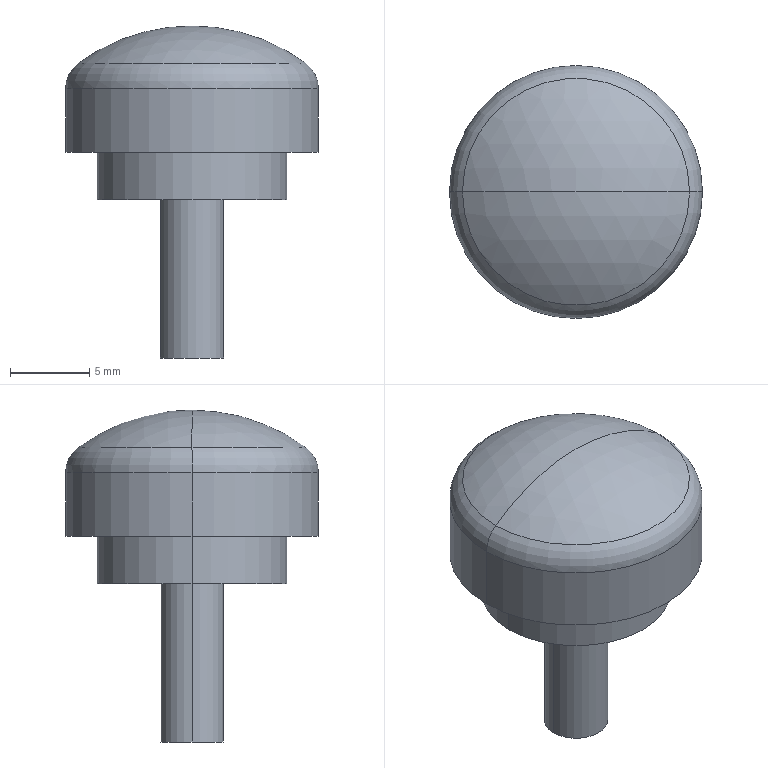Part | SolidWorks | features ICE 2, Dome 1, Extrusion 1, Fillet 1 | 1 solid | 13 faces | box 16 x 16 x 21 mm | volume 1779 mm3 | cylinder 6 | plane 3 | torus 2 | sphere 2 | commonest cylinder face diameters 4 x2 12 x2 16 x2
STEP:
#1=CARTESIAN_POINT('',(7.18,0.,18.655));
#2=VERTEX_POINT('',#1);
#3=CARTESIAN_POINT('',(-7.18,0.,18.655));
#4=VERTEX_POINT('',#3);
#5=CARTESIAN_POINT('',(0.,0.,18.655));
#6=DIRECTION('',(0.,0.,1.));
#7=DIRECTION('',(-1.,0.,0.));
#8=AXIS2_PLACEMENT_3D('',#5,#6,#7);
#9=CIRCLE('',#8,7.18);
#10=EDGE_CURVE('',#2,#4,#9,.T.);
#11=ORIENTED_EDGE('',*,*,#10,.F.);
#12=CARTESIAN_POINT('',(8.,0.,17.041));
#13=VERTEX_POINT('',#12);
#14=CARTESIAN_POINT('',(6.,0.,17.041));
#15=DIRECTION('',(0.,1.,0.));
#16=DIRECTION('',(-1.,0.,0.));
#17=AXIS2_PLACEMENT_3D('',#14,#15,#16);
#18=CIRCLE('',#17,2.);
#19=EDGE_CURVE('',#2,#13,#18,.T.);
#20=ORIENTED_EDGE('',*,*,#19,.T.);
#21=CARTESIAN_POINT('',(-8.,0.,17.041));
#22=VERTEX_POINT('',#21);
#23=CARTESIAN_POINT('',(0.,0.,17.041));
#24=DIRECTION('',(0.,0.,-1.));
#25=DIRECTION('',(-1.,0.,0.));
#26=AXIS2_PLACEMENT_3D('',#23,#24,#25);
#27=CIRCLE('',#26,8.);
#28=EDGE_CURVE('',#22,#13,#27,.T.);
#29=ORIENTED_EDGE('',*,*,#28,.F.);
#30=CARTESIAN_POINT('',(-6.,0.,17.041));
#31=DIRECTION('',(0.,-1.,0.));
#32=DIRECTION('',(0.,0.,-1.));
#33=AXIS2_PLACEMENT_3D('',#30,#31,#32);
#34=CIRCLE('',#33,2.);
#35=EDGE_CURVE('',#4,#22,#34,.T.);
#36=ORIENTED_EDGE('',*,*,#35,.F.);
#37=EDGE_LOOP('',(#11,#20,#29,#36));
#38=FACE_OUTER_BOUND('',#37,.T.);
#39=CARTESIAN_POINT('',(0.,0.,17.041));
#40=DIRECTION('',(0.,0.,-1.));
#41=DIRECTION('',(-1.,0.,0.));
#42=AXIS2_PLACEMENT_3D('',#39,#40,#41);
#43=TOROIDAL_SURFACE('',#42,6.,2.);
#44=ADVANCED_FACE('',(#38),#43,.T.);
#45=ORIENTED_EDGE('',*,*,#28,.T.);
#46=CARTESIAN_POINT('',(8.,0.,13.));
#47=VERTEX_POINT('',#46);
#48=CARTESIAN_POINT('',(8.,0.,18.));
#49=DIRECTION('',(0.,0.,-1.));
#50=VECTOR('',#49,1000.);
#51=LINE('',#48,#50);
#52=EDGE_CURVE('',#13,#47,#51,.T.);
#53=ORIENTED_EDGE('',*,*,#52,.T.);
#54=CARTESIAN_POINT('',(-8.,0.,13.));
#55=VERTEX_POINT('',#54);
#56=CARTESIAN_POINT('',(0.,0.,13.));
#57=DIRECTION('',(0.,0.,-1.));
#58=DIRECTION('',(-1.,0.,0.));
#59=AXIS2_PLACEMENT_3D('',#56,#57,#58);
#60=CIRCLE('',#59,8.);
#61=EDGE_CURVE('',#55,#47,#60,.T.);
#62=ORIENTED_EDGE('',*,*,#61,.F.);
#63=CARTESIAN_POINT('',(-8.,0.,18.));
#64=DIRECTION('',(0.,0.,-1.));
#65=VECTOR('',#64,1000.);
#66=LINE('',#63,#65);
#67=EDGE_CURVE('',#22,#55,#66,.T.);
#68=ORIENTED_EDGE('',*,*,#67,.F.);
#69=EDGE_LOOP('',(#45,#53,#62,#68));
#70=FACE_OUTER_BOUND('',#69,.T.);
#71=CARTESIAN_POINT('',(0.,0.,18.));
#72=DIRECTION('',(0.,0.,-1.));
#73=DIRECTION('',(-1.,0.,0.));
#74=AXIS2_PLACEMENT_3D('',#71,#72,#73);
#75=CYLINDRICAL_SURFACE('',#74,8.);
#76=ADVANCED_FACE('',(#70),#75,.T.);
#77=ORIENTED_EDGE('',*,*,#10,.T.);
#78=CARTESIAN_POINT('',(0.,0.,21.));
#79=VERTEX_POINT('',#78);
#80=CARTESIAN_POINT('',(0.,0.,8.833));
#81=DIRECTION('',(0.,1.,0.));
#82=DIRECTION('',(-1.,0.,0.));
#83=AXIS2_PLACEMENT_3D('',#80,#81,#82);
#84=CIRCLE('',#83,12.167);
#85=EDGE_CURVE('',#4,#79,#84,.T.);
#86=ORIENTED_EDGE('',*,*,#85,.T.);
#87=CARTESIAN_POINT('',(0.,0.,8.833));
#88=DIRECTION('',(0.,-1.,0.));
#89=DIRECTION('',(0.,0.,-1.));
#90=AXIS2_PLACEMENT_3D('',#87,#88,#89);
#91=CIRCLE('',#90,12.167);
#92=EDGE_CURVE('',#2,#79,#91,.T.);
#93=ORIENTED_EDGE('',*,*,#92,.F.);
#94=EDGE_LOOP('',(#77,#86,#93));
#95=FACE_OUTER_BOUND('',#94,.T.);
#96=CARTESIAN_POINT('',(0.,0.,8.833));
#97=DIRECTION('',(0.,1.,0.));
#98=DIRECTION('',(1.,0.,0.));
#99=AXIS2_PLACEMENT_3D('',#96,#97,#98);
#100=SPHERICAL_SURFACE('',#99,12.167);
#101=ADVANCED_FACE('',(#95),#100,.T.);
#102=CARTESIAN_POINT('',(-6.,0.,13.));
#103=VERTEX_POINT('',#102);
#104=CARTESIAN_POINT('',(6.,0.,13.));
#105=VERTEX_POINT('',#104);
#106=CARTESIAN_POINT('',(0.,0.,13.));
#107=DIRECTION('',(0.,0.,-1.));
#108=DIRECTION('',(-1.,0.,0.));
#109=AXIS2_PLACEMENT_3D('',#106,#107,#108);
#110=CIRCLE('',#109,6.);
#111=EDGE_CURVE('',#103,#105,#110,.T.);
#112=ORIENTED_EDGE('',*,*,#111,.T.);
#113=CARTESIAN_POINT('',(6.,0.,10.));
#114=VERTEX_POINT('',#113);
#115=CARTESIAN_POINT('',(6.,0.,13.));
#116=DIRECTION('',(0.,0.,-1.));
#117=VECTOR('',#116,1000.);
#118=LINE('',#115,#117);
#119=EDGE_CURVE('',#105,#114,#118,.T.);
#120=ORIENTED_EDGE('',*,*,#119,.T.);
#121=CARTESIAN_POINT('',(-6.,0.,10.));
#122=VERTEX_POINT('',#121);
#123=CARTESIAN_POINT('',(0.,0.,10.));
#124=DIRECTION('',(0.,0.,-1.));
#125=DIRECTION('',(-1.,0.,0.));
#126=AXIS2_PLACEMENT_3D('',#123,#124,#125);
#127=CIRCLE('',#126,6.);
#128=EDGE_CURVE('',#122,#114,#127,.T.);
#129=ORIENTED_EDGE('',*,*,#128,.F.);
#130=CARTESIAN_POINT('',(-6.,0.,13.));
#131=DIRECTION('',(0.,0.,-1.));
#132=VECTOR('',#131,1000.);
#133=LINE('',#130,#132);
#134=EDGE_CURVE('',#103,#122,#133,.T.);
#135=ORIENTED_EDGE('',*,*,#134,.F.);
#136=EDGE_LOOP('',(#112,#120,#129,#135));
#137=FACE_OUTER_BOUND('',#136,.T.);
#138=CARTESIAN_POINT('',(0.,0.,13.));
#139=DIRECTION('',(0.,0.,-1.));
#140=DIRECTION('',(-1.,0.,0.));
#141=AXIS2_PLACEMENT_3D('',#138,#139,#140);
#142=CYLINDRICAL_SURFACE('',#141,6.);
#143=ADVANCED_FACE('',(#137),#142,.T.);
#144=CARTESIAN_POINT('',(2.,0.,10.));
#145=VERTEX_POINT('',#144);
#146=CARTESIAN_POINT('',(-2.,0.,10.));
#147=VERTEX_POINT('',#146);
#148=CARTESIAN_POINT('',(0.,0.,10.));
#149=DIRECTION('',(0.,0.,1.));
#150=DIRECTION('',(1.,0.,0.));
#151=AXIS2_PLACEMENT_3D('',#148,#149,#150);
#152=CIRCLE('',#151,2.);
#153=EDGE_CURVE('',#145,#147,#152,.T.);
#154=ORIENTED_EDGE('',*,*,#153,.F.);
#155=CARTESIAN_POINT('',(2.,0.,0.));
#156=VERTEX_POINT('',#155);
#157=CARTESIAN_POINT('',(2.,0.,10.));
#158=DIRECTION('',(0.,0.,-1.));
#159=VECTOR('',#158,1000.);
#160=LINE('',#157,#159);
#161=EDGE_CURVE('',#145,#156,#160,.T.);
#162=ORIENTED_EDGE('',*,*,#161,.T.);
#163=CARTESIAN_POINT('',(-2.,0.,0.));
#164=VERTEX_POINT('',#163);
#165=CARTESIAN_POINT('',(0.,0.,0.));
#166=DIRECTION('',(0.,0.,1.));
#167=DIRECTION('',(1.,0.,0.));
#168=AXIS2_PLACEMENT_3D('',#165,#166,#167);
#169=CIRCLE('',#168,2.);
#170=EDGE_CURVE('',#156,#164,#169,.T.);
#171=ORIENTED_EDGE('',*,*,#170,.T.);
#172=CARTESIAN_POINT('',(-2.,0.,10.));
#173=DIRECTION('',(0.,0.,-1.));
#174=VECTOR('',#173,1000.);
#175=LINE('',#172,#174);
#176=EDGE_CURVE('',#147,#164,#175,.T.);
#177=ORIENTED_EDGE('',*,*,#176,.F.);
#178=EDGE_LOOP('',(#154,#162,#171,#177));
#179=FACE_OUTER_BOUND('',#178,.T.);
#180=CARTESIAN_POINT('',(0.,0.,10.));
#181=DIRECTION('',(0.,0.,-1.));
#182=DIRECTION('',(-1.,0.,0.));
#183=AXIS2_PLACEMENT_3D('',#180,#181,#182);
#184=CYLINDRICAL_SURFACE('',#183,2.);
#185=ADVANCED_FACE('',(#179),#184,.T.);
#186=CARTESIAN_POINT('',(0.,0.,10.));
#187=DIRECTION('',(0.,0.,1.));
#188=DIRECTION('',(1.,0.,0.));
#189=AXIS2_PLACEMENT_3D('',#186,#187,#188);
#190=CIRCLE('',#189,2.);
#191=EDGE_CURVE('',#147,#145,#190,.T.);
#192=ORIENTED_EDGE('',*,*,#191,.T.);
#193=ORIENTED_EDGE('',*,*,#153,.T.);
#194=EDGE_LOOP('',(#192,#193));
#195=FACE_BOUND('',#194,.T.);
#196=ORIENTED_EDGE('',*,*,#128,.T.);
#197=CARTESIAN_POINT('',(0.,0.,10.));
#198=DIRECTION('',(0.,0.,-1.));
#199=DIRECTION('',(-1.,0.,0.));
#200=AXIS2_PLACEMENT_3D('',#197,#198,#199);
#201=CIRCLE('',#200,6.);
#202=EDGE_CURVE('',#114,#122,#201,.T.);
#203=ORIENTED_EDGE('',*,*,#202,.T.);
#204=EDGE_LOOP('',(#196,#203));
#205=FACE_OUTER_BOUND('',#204,.T.);
#206=CARTESIAN_POINT('',(0.,0.,10.));
#207=DIRECTION('',(0.,0.,1.));
#208=DIRECTION('',(1.,0.,0.));
#209=AXIS2_PLACEMENT_3D('',#206,#207,#208);
#210=PLANE('',#209);
#211=ADVANCED_FACE('',(#195,#205),#210,.F.);
#212=ORIENTED_EDGE('',*,*,#161,.F.);
#213=ORIENTED_EDGE('',*,*,#191,.F.);
#214=ORIENTED_EDGE('',*,*,#176,.T.);
#215=CARTESIAN_POINT('',(0.,0.,0.));
#216=DIRECTION('',(0.,0.,1.));
#217=DIRECTION('',(1.,0.,0.));
#218=AXIS2_PLACEMENT_3D('',#215,#216,#217);
#219=CIRCLE('',#218,2.);
#220=EDGE_CURVE('',#164,#156,#219,.T.);
#221=ORIENTED_EDGE('',*,*,#220,.T.);
#222=EDGE_LOOP('',(#212,#213,#214,#221));
#223=FACE_OUTER_BOUND('',#222,.T.);
#224=CARTESIAN_POINT('',(0.,0.,10.));
#225=DIRECTION('',(0.,0.,-1.));
#226=DIRECTION('',(-1.,0.,0.));
#227=AXIS2_PLACEMENT_3D('',#224,#225,#226);
#228=CYLINDRICAL_SURFACE('',#227,2.);
#229=ADVANCED_FACE('',(#223),#228,.T.);
#230=ORIENTED_EDGE('',*,*,#220,.F.);
#231=ORIENTED_EDGE('',*,*,#170,.F.);
#232=EDGE_LOOP('',(#230,#231));
#233=FACE_OUTER_BOUND('',#232,.T.);
#234=CARTESIAN_POINT('',(0.,0.,0.));
#235=DIRECTION('',(0.,0.,1.));
#236=DIRECTION('',(1.,0.,0.));
#237=AXIS2_PLACEMENT_3D('',#234,#235,#236);
#238=PLANE('',#237);
#239=ADVANCED_FACE('',(#233),#238,.F.);
#240=ORIENTED_EDGE('',*,*,#111,.F.);
#241=CARTESIAN_POINT('',(0.,0.,13.));
#242=DIRECTION('',(0.,0.,-1.));
#243=DIRECTION('',(-1.,0.,0.));
#244=AXIS2_PLACEMENT_3D('',#241,#242,#243);
#245=CIRCLE('',#244,6.);
#246=EDGE_CURVE('',#105,#103,#245,.T.);
#247=ORIENTED_EDGE('',*,*,#246,.F.);
#248=EDGE_LOOP('',(#240,#247));
#249=FACE_BOUND('',#248,.T.);
#250=ORIENTED_EDGE('',*,*,#61,.T.);
#251=CARTESIAN_POINT('',(0.,0.,13.));
#252=DIRECTION('',(0.,0.,-1.));
#253=DIRECTION('',(-1.,0.,0.));
#254=AXIS2_PLACEMENT_3D('',#251,#252,#253);
#255=CIRCLE('',#254,8.);
#256=EDGE_CURVE('',#47,#55,#255,.T.);
#257=ORIENTED_EDGE('',*,*,#256,.T.);
#258=EDGE_LOOP('',(#250,#257));
#259=FACE_OUTER_BOUND('',#258,.T.);
#260=CARTESIAN_POINT('',(0.,0.,13.));
#261=DIRECTION('',(0.,0.,-1.));
#262=DIRECTION('',(-1.,0.,0.));
#263=AXIS2_PLACEMENT_3D('',#260,#261,#262);
#264=PLANE('',#263);
#265=ADVANCED_FACE('',(#249,#259),#264,.T.);
#266=ORIENTED_EDGE('',*,*,#119,.F.);
#267=ORIENTED_EDGE('',*,*,#246,.T.);
#268=ORIENTED_EDGE('',*,*,#134,.T.);
#269=ORIENTED_EDGE('',*,*,#202,.F.);
#270=EDGE_LOOP('',(#266,#267,#268,#269));
#271=FACE_OUTER_BOUND('',#270,.T.);
#272=CARTESIAN_POINT('',(0.,0.,13.));
#273=DIRECTION('',(0.,0.,-1.));
#274=DIRECTION('',(-1.,0.,0.));
#275=AXIS2_PLACEMENT_3D('',#272,#273,#274);
#276=CYLINDRICAL_SURFACE('',#275,6.);
#277=ADVANCED_FACE('',(#271),#276,.T.);
#278=ORIENTED_EDGE('',*,*,#85,.F.);
#279=CARTESIAN_POINT('',(0.,0.,18.655));
#280=DIRECTION('',(0.,0.,1.));
#281=DIRECTION('',(-1.,0.,0.));
#282=AXIS2_PLACEMENT_3D('',#279,#280,#281);
#283=CIRCLE('',#282,7.18);
#284=EDGE_CURVE('',#4,#2,#283,.T.);
#285=ORIENTED_EDGE('',*,*,#284,.T.);
#286=ORIENTED_EDGE('',*,*,#92,.T.);
#287=EDGE_LOOP('',(#278,#285,#286));
#288=FACE_OUTER_BOUND('',#287,.T.);
#289=CARTESIAN_POINT('',(0.,0.,8.833));
#290=DIRECTION('',(0.,1.,0.));
#291=DIRECTION('',(1.,0.,0.));
#292=AXIS2_PLACEMENT_3D('',#289,#290,#291);
#293=SPHERICAL_SURFACE('',#292,12.167);
#294=ADVANCED_FACE('',(#288),#293,.T.);
#295=ORIENTED_EDGE('',*,*,#52,.F.);
#296=CARTESIAN_POINT('',(0.,0.,17.041));
#297=DIRECTION('',(0.,0.,-1.));
#298=DIRECTION('',(-1.,0.,0.));
#299=AXIS2_PLACEMENT_3D('',#296,#297,#298);
#300=CIRCLE('',#299,8.);
#301=EDGE_CURVE('',#13,#22,#300,.T.);
#302=ORIENTED_EDGE('',*,*,#301,.T.);
#303=ORIENTED_EDGE('',*,*,#67,.T.);
#304=ORIENTED_EDGE('',*,*,#256,.F.);
#305=EDGE_LOOP('',(#295,#302,#303,#304));
#306=FACE_OUTER_BOUND('',#305,.T.);
#307=CARTESIAN_POINT('',(0.,0.,18.));
#308=DIRECTION('',(0.,0.,-1.));
#309=DIRECTION('',(-1.,0.,0.));
#310=AXIS2_PLACEMENT_3D('',#307,#308,#309);
#311=CYLINDRICAL_SURFACE('',#310,8.);
#312=ADVANCED_FACE('',(#306),#311,.T.);
#313=ORIENTED_EDGE('',*,*,#19,.F.);
#314=ORIENTED_EDGE('',*,*,#284,.F.);
#315=ORIENTED_EDGE('',*,*,#35,.T.);
#316=ORIENTED_EDGE('',*,*,#301,.F.);
#317=EDGE_LOOP('',(#313,#314,#315,#316));
#318=FACE_OUTER_BOUND('',#317,.T.);
#319=CARTESIAN_POINT('',(0.,0.,17.041));
#320=DIRECTION('',(0.,0.,-1.));
#321=DIRECTION('',(-1.,0.,0.));
#322=AXIS2_PLACEMENT_3D('',#319,#320,#321);
#323=TOROIDAL_SURFACE('',#322,6.,2.);
#324=ADVANCED_FACE('',(#318),#323,.T.);
#325=CLOSED_SHELL('',(#44,#76,#101,#143,#185,#211,#229,#239,#265,#277,#294,#312,#324));
#326=MANIFOLD_SOLID_BREP('',#325);
#327=CARTESIAN_POINT('',(0.,0.,0.));
#328=DIRECTION('',(0.,0.,1.));
#329=DIRECTION('',(1.,0.,0.));
#330=AXIS2_PLACEMENT_3D('',#327,#328,#329);
#331=(LENGTH_UNIT()NAMED_UNIT(*)SI_UNIT(.MILLI.,.METRE.));
#332=UNCERTAINTY_MEASURE_WITH_UNIT(LENGTH_MEASURE(0.00001),#331,'','');
#333=(NAMED_UNIT(*)PLANE_ANGLE_UNIT()SI_UNIT($,.RADIAN.));
#334=(NAMED_UNIT(*)SI_UNIT($,.STERADIAN.)SOLID_ANGLE_UNIT());
#335=(GEOMETRIC_REPRESENTATION_CONTEXT(3)GLOBAL_UNCERTAINTY_ASSIGNED_CONTEXT((#332))GLOBAL_UNIT_ASSIGNED_CONTEXT((#331,#333,#334))REPRESENTATION_CONTEXT('',''));
#336=ADVANCED_BREP_SHAPE_REPRESENTATION('',(#326,#330),#335);